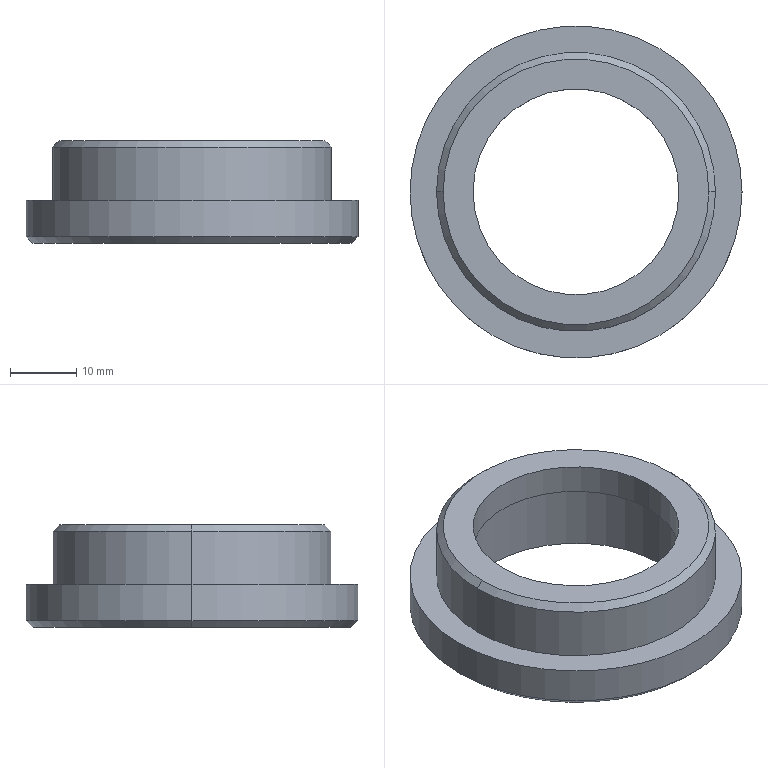Part | SolidWorks | features ICE 4, Chamfer 1, Extrusion 1 | 1 solid | 19 faces | box 50 x 50 x 15.5 mm | volume 11056 mm3 | cylinder 10 | plane 5 | cone 4 | commonest cylinder face diameters 31 x2 33 x2 35 x2 42 x2 50 x2
STEP:
#1=CARTESIAN_POINT('',(-24.,0.,0.));
#2=VERTEX_POINT('',#1);
#3=CARTESIAN_POINT('',(24.,0.,0.));
#4=VERTEX_POINT('',#3);
#5=CARTESIAN_POINT('',(0.,0.,0.));
#6=DIRECTION('',(0.,0.,-1.));
#7=DIRECTION('',(1.,0.,0.));
#8=AXIS2_PLACEMENT_3D('',#5,#6,#7);
#9=CIRCLE('',#8,24.);
#10=EDGE_CURVE('',#2,#4,#9,.T.);
#11=ORIENTED_EDGE('',*,*,#10,.F.);
#12=CARTESIAN_POINT('',(-25.,0.,1.));
#13=VERTEX_POINT('',#12);
#14=CARTESIAN_POINT('',(-25.,0.,1.));
#15=DIRECTION('',(-0.7071,0.,0.7071));
#16=VECTOR('',#15,1000.);
#17=LINE('',#14,#16);
#18=EDGE_CURVE('',#2,#13,#17,.T.);
#19=ORIENTED_EDGE('',*,*,#18,.T.);
#20=CARTESIAN_POINT('',(25.,0.,1.));
#21=VERTEX_POINT('',#20);
#22=CARTESIAN_POINT('',(0.,0.,1.));
#23=DIRECTION('',(0.,0.,1.));
#24=DIRECTION('',(1.,0.,0.));
#25=AXIS2_PLACEMENT_3D('',#22,#23,#24);
#26=CIRCLE('',#25,25.);
#27=EDGE_CURVE('',#21,#13,#26,.T.);
#28=ORIENTED_EDGE('',*,*,#27,.F.);
#29=CARTESIAN_POINT('',(25.,0.,1.));
#30=DIRECTION('',(0.7071,0.,0.7071));
#31=VECTOR('',#30,1000.);
#32=LINE('',#29,#31);
#33=EDGE_CURVE('',#4,#21,#32,.T.);
#34=ORIENTED_EDGE('',*,*,#33,.F.);
#35=EDGE_LOOP('',(#11,#19,#28,#34));
#36=FACE_OUTER_BOUND('',#35,.T.);
#37=CARTESIAN_POINT('',(0.,0.,1.));
#38=DIRECTION('',(0.,0.,1.));
#39=DIRECTION('',(1.,0.,0.));
#40=AXIS2_PLACEMENT_3D('',#37,#38,#39);
#41=CONICAL_SURFACE('',#40,25.,0.7854);
#42=ADVANCED_FACE('',(#36),#41,.T.);
#43=CARTESIAN_POINT('',(20.,0.,15.5));
#44=VERTEX_POINT('',#43);
#45=CARTESIAN_POINT('',(-20.,0.,15.5));
#46=VERTEX_POINT('',#45);
#47=CARTESIAN_POINT('',(0.,0.,15.5));
#48=DIRECTION('',(0.,0.,1.));
#49=DIRECTION('',(1.,0.,0.));
#50=AXIS2_PLACEMENT_3D('',#47,#48,#49);
#51=CIRCLE('',#50,20.);
#52=EDGE_CURVE('',#44,#46,#51,.T.);
#53=ORIENTED_EDGE('',*,*,#52,.F.);
#54=CARTESIAN_POINT('',(21.,0.,14.5));
#55=VERTEX_POINT('',#54);
#56=CARTESIAN_POINT('',(20.,0.,15.5));
#57=DIRECTION('',(0.7071,0.,-0.7071));
#58=VECTOR('',#57,1000.);
#59=LINE('',#56,#58);
#60=EDGE_CURVE('',#44,#55,#59,.T.);
#61=ORIENTED_EDGE('',*,*,#60,.T.);
#62=CARTESIAN_POINT('',(-21.,0.,14.5));
#63=VERTEX_POINT('',#62);
#64=CARTESIAN_POINT('',(0.,0.,14.5));
#65=DIRECTION('',(0.,0.,-1.));
#66=DIRECTION('',(1.,0.,0.));
#67=AXIS2_PLACEMENT_3D('',#64,#65,#66);
#68=CIRCLE('',#67,21.);
#69=EDGE_CURVE('',#63,#55,#68,.T.);
#70=ORIENTED_EDGE('',*,*,#69,.F.);
#71=CARTESIAN_POINT('',(-20.,0.,15.5));
#72=DIRECTION('',(-0.7071,0.,-0.7071));
#73=VECTOR('',#72,1000.);
#74=LINE('',#71,#73);
#75=EDGE_CURVE('',#46,#63,#74,.T.);
#76=ORIENTED_EDGE('',*,*,#75,.F.);
#77=EDGE_LOOP('',(#53,#61,#70,#76));
#78=FACE_OUTER_BOUND('',#77,.T.);
#79=CARTESIAN_POINT('',(0.,0.,15.5));
#80=DIRECTION('',(0.,0.,-1.));
#81=DIRECTION('',(-1.,0.,0.));
#82=AXIS2_PLACEMENT_3D('',#79,#80,#81);
#83=CONICAL_SURFACE('',#82,20.,0.7854);
#84=ADVANCED_FACE('',(#78),#83,.T.);
#85=CARTESIAN_POINT('',(-16.5,0.,11.5));
#86=VERTEX_POINT('',#85);
#87=CARTESIAN_POINT('',(16.5,0.,11.5));
#88=VERTEX_POINT('',#87);
#89=CARTESIAN_POINT('',(0.,0.,11.5));
#90=DIRECTION('',(0.,0.,-1.));
#91=DIRECTION('',(-1.,0.,0.));
#92=AXIS2_PLACEMENT_3D('',#89,#90,#91);
#93=CIRCLE('',#92,16.5);
#94=EDGE_CURVE('',#86,#88,#93,.T.);
#95=ORIENTED_EDGE('',*,*,#94,.T.);
#96=CARTESIAN_POINT('',(16.5,0.,11.));
#97=VERTEX_POINT('',#96);
#98=CARTESIAN_POINT('',(16.5,0.,11.5));
#99=DIRECTION('',(0.,0.,-1.));
#100=VECTOR('',#99,1000.);
#101=LINE('',#98,#100);
#102=EDGE_CURVE('',#88,#97,#101,.T.);
#103=ORIENTED_EDGE('',*,*,#102,.T.);
#104=CARTESIAN_POINT('',(-16.5,0.,11.));
#105=VERTEX_POINT('',#104);
#106=CARTESIAN_POINT('',(0.,0.,11.));
#107=DIRECTION('',(0.,0.,-1.));
#108=DIRECTION('',(-1.,0.,0.));
#109=AXIS2_PLACEMENT_3D('',#106,#107,#108);
#110=CIRCLE('',#109,16.5);
#111=EDGE_CURVE('',#105,#97,#110,.T.);
#112=ORIENTED_EDGE('',*,*,#111,.F.);
#113=CARTESIAN_POINT('',(-16.5,0.,11.5));
#114=DIRECTION('',(0.,0.,-1.));
#115=VECTOR('',#114,1000.);
#116=LINE('',#113,#115);
#117=EDGE_CURVE('',#86,#105,#116,.T.);
#118=ORIENTED_EDGE('',*,*,#117,.F.);
#119=EDGE_LOOP('',(#95,#103,#112,#118));
#120=FACE_OUTER_BOUND('',#119,.T.);
#121=CARTESIAN_POINT('',(0.,0.,11.5));
#122=DIRECTION('',(0.,0.,-1.));
#123=DIRECTION('',(-1.,0.,0.));
#124=AXIS2_PLACEMENT_3D('',#121,#122,#123);
#125=CYLINDRICAL_SURFACE('',#124,16.5);
#126=ADVANCED_FACE('',(#120),#125,.T.);
#127=CARTESIAN_POINT('',(17.5,0.,11.5));
#128=VERTEX_POINT('',#127);
#129=CARTESIAN_POINT('',(-17.5,0.,11.5));
#130=VERTEX_POINT('',#129);
#131=CARTESIAN_POINT('',(0.,0.,11.5));
#132=DIRECTION('',(0.,0.,-1.));
#133=DIRECTION('',(-1.,0.,0.));
#134=AXIS2_PLACEMENT_3D('',#131,#132,#133);
#135=CIRCLE('',#134,17.5);
#136=EDGE_CURVE('',#128,#130,#135,.T.);
#137=ORIENTED_EDGE('',*,*,#136,.F.);
#138=CARTESIAN_POINT('',(17.5,0.,0.));
#139=VERTEX_POINT('',#138);
#140=CARTESIAN_POINT('',(17.5,0.,11.));
#141=DIRECTION('',(0.,0.,-1.));
#142=VECTOR('',#141,1000.);
#143=LINE('',#140,#142);
#144=EDGE_CURVE('',#128,#139,#143,.T.);
#145=ORIENTED_EDGE('',*,*,#144,.T.);
#146=CARTESIAN_POINT('',(-17.5,0.,0.));
#147=VERTEX_POINT('',#146);
#148=CARTESIAN_POINT('',(0.,0.,0.));
#149=DIRECTION('',(0.,0.,-1.));
#150=DIRECTION('',(-1.,0.,0.));
#151=AXIS2_PLACEMENT_3D('',#148,#149,#150);
#152=CIRCLE('',#151,17.5);
#153=EDGE_CURVE('',#139,#147,#152,.T.);
#154=ORIENTED_EDGE('',*,*,#153,.T.);
#155=CARTESIAN_POINT('',(-17.5,0.,11.));
#156=DIRECTION('',(0.,0.,-1.));
#157=VECTOR('',#156,1000.);
#158=LINE('',#155,#157);
#159=EDGE_CURVE('',#130,#147,#158,.T.);
#160=ORIENTED_EDGE('',*,*,#159,.F.);
#161=EDGE_LOOP('',(#137,#145,#154,#160));
#162=FACE_OUTER_BOUND('',#161,.T.);
#163=CARTESIAN_POINT('',(0.,0.,11.));
#164=DIRECTION('',(0.,0.,-1.));
#165=DIRECTION('',(-1.,0.,0.));
#166=AXIS2_PLACEMENT_3D('',#163,#164,#165);
#167=CYLINDRICAL_SURFACE('',#166,17.5);
#168=ADVANCED_FACE('',(#162),#167,.F.);
#169=ORIENTED_EDGE('',*,*,#69,.T.);
#170=CARTESIAN_POINT('',(21.,0.,6.5));
#171=VERTEX_POINT('',#170);
#172=CARTESIAN_POINT('',(21.,0.,15.5));
#173=DIRECTION('',(0.,0.,-1.));
#174=VECTOR('',#173,1000.);
#175=LINE('',#172,#174);
#176=EDGE_CURVE('',#55,#171,#175,.T.);
#177=ORIENTED_EDGE('',*,*,#176,.T.);
#178=CARTESIAN_POINT('',(-21.,0.,6.5));
#179=VERTEX_POINT('',#178);
#180=CARTESIAN_POINT('',(0.,0.,6.5));
#181=DIRECTION('',(0.,0.,1.));
#182=DIRECTION('',(1.,0.,0.));
#183=AXIS2_PLACEMENT_3D('',#180,#181,#182);
#184=CIRCLE('',#183,21.);
#185=EDGE_CURVE('',#171,#179,#184,.T.);
#186=ORIENTED_EDGE('',*,*,#185,.T.);
#187=CARTESIAN_POINT('',(-21.,0.,15.5));
#188=DIRECTION('',(0.,0.,-1.));
#189=VECTOR('',#188,1000.);
#190=LINE('',#187,#189);
#191=EDGE_CURVE('',#63,#179,#190,.T.);
#192=ORIENTED_EDGE('',*,*,#191,.F.);
#193=EDGE_LOOP('',(#169,#177,#186,#192));
#194=FACE_OUTER_BOUND('',#193,.T.);
#195=CARTESIAN_POINT('',(0.,0.,15.5));
#196=DIRECTION('',(0.,0.,-1.));
#197=DIRECTION('',(-1.,0.,0.));
#198=AXIS2_PLACEMENT_3D('',#195,#196,#197);
#199=CYLINDRICAL_SURFACE('',#198,21.);
#200=ADVANCED_FACE('',(#194),#199,.T.);
#201=CARTESIAN_POINT('',(25.,0.,6.5));
#202=VERTEX_POINT('',#201);
#203=CARTESIAN_POINT('',(-25.,0.,6.5));
#204=VERTEX_POINT('',#203);
#205=CARTESIAN_POINT('',(0.,0.,6.5));
#206=DIRECTION('',(0.,0.,1.));
#207=DIRECTION('',(1.,0.,0.));
#208=AXIS2_PLACEMENT_3D('',#205,#206,#207);
#209=CIRCLE('',#208,25.);
#210=EDGE_CURVE('',#202,#204,#209,.T.);
#211=ORIENTED_EDGE('',*,*,#210,.F.);
#212=CARTESIAN_POINT('',(25.,0.,6.5));
#213=DIRECTION('',(0.,0.,-1.));
#214=VECTOR('',#213,1000.);
#215=LINE('',#212,#214);
#216=EDGE_CURVE('',#202,#21,#215,.T.);
#217=ORIENTED_EDGE('',*,*,#216,.T.);
#218=ORIENTED_EDGE('',*,*,#27,.T.);
#219=CARTESIAN_POINT('',(-25.,0.,6.5));
#220=DIRECTION('',(0.,0.,-1.));
#221=VECTOR('',#220,1000.);
#222=LINE('',#219,#221);
#223=EDGE_CURVE('',#204,#13,#222,.T.);
#224=ORIENTED_EDGE('',*,*,#223,.F.);
#225=EDGE_LOOP('',(#211,#217,#218,#224));
#226=FACE_OUTER_BOUND('',#225,.T.);
#227=CARTESIAN_POINT('',(0.,0.,6.5));
#228=DIRECTION('',(0.,0.,-1.));
#229=DIRECTION('',(-1.,0.,0.));
#230=AXIS2_PLACEMENT_3D('',#227,#228,#229);
#231=CYLINDRICAL_SURFACE('',#230,25.);
#232=ADVANCED_FACE('',(#226),#231,.T.);
#233=CARTESIAN_POINT('',(-15.5,0.,11.));
#234=VERTEX_POINT('',#233);
#235=CARTESIAN_POINT('',(15.5,0.,11.));
#236=VERTEX_POINT('',#235);
#237=CARTESIAN_POINT('',(0.,0.,11.));
#238=DIRECTION('',(0.,0.,1.));
#239=DIRECTION('',(-1.,0.,0.));
#240=AXIS2_PLACEMENT_3D('',#237,#238,#239);
#241=CIRCLE('',#240,15.5);
#242=EDGE_CURVE('',#234,#236,#241,.T.);
#243=ORIENTED_EDGE('',*,*,#242,.F.);
#244=CARTESIAN_POINT('',(-15.5,0.,15.5));
#245=VERTEX_POINT('',#244);
#246=CARTESIAN_POINT('',(-15.5,0.,-27.5));
#247=DIRECTION('',(0.,0.,1.));
#248=VECTOR('',#247,1000.);
#249=LINE('',#246,#248);
#250=EDGE_CURVE('',#234,#245,#249,.T.);
#251=ORIENTED_EDGE('',*,*,#250,.T.);
#252=CARTESIAN_POINT('',(15.5,0.,15.5));
#253=VERTEX_POINT('',#252);
#254=CARTESIAN_POINT('',(0.,0.,15.5));
#255=DIRECTION('',(0.,0.,1.));
#256=DIRECTION('',(1.,0.,0.));
#257=AXIS2_PLACEMENT_3D('',#254,#255,#256);
#258=CIRCLE('',#257,15.5);
#259=EDGE_CURVE('',#245,#253,#258,.T.);
#260=ORIENTED_EDGE('',*,*,#259,.T.);
#261=CARTESIAN_POINT('',(15.5,0.,-27.5));
#262=DIRECTION('',(0.,0.,1.));
#263=VECTOR('',#262,1000.);
#264=LINE('',#261,#263);
#265=EDGE_CURVE('',#236,#253,#264,.T.);
#266=ORIENTED_EDGE('',*,*,#265,.F.);
#267=EDGE_LOOP('',(#243,#251,#260,#266));
#268=FACE_OUTER_BOUND('',#267,.T.);
#269=CARTESIAN_POINT('',(0.,0.,-27.5));
#270=DIRECTION('',(0.,0.,1.));
#271=DIRECTION('',(1.,0.,0.));
#272=AXIS2_PLACEMENT_3D('',#269,#270,#271);
#273=CYLINDRICAL_SURFACE('',#272,15.5);
#274=ADVANCED_FACE('',(#268),#273,.F.);
#275=CARTESIAN_POINT('',(0.,0.,11.));
#276=DIRECTION('',(0.,0.,1.));
#277=DIRECTION('',(-1.,0.,0.));
#278=AXIS2_PLACEMENT_3D('',#275,#276,#277);
#279=CIRCLE('',#278,15.5);
#280=EDGE_CURVE('',#236,#234,#279,.T.);
#281=ORIENTED_EDGE('',*,*,#280,.T.);
#282=ORIENTED_EDGE('',*,*,#242,.T.);
#283=EDGE_LOOP('',(#281,#282));
#284=FACE_BOUND('',#283,.T.);
#285=ORIENTED_EDGE('',*,*,#111,.T.);
#286=CARTESIAN_POINT('',(0.,0.,11.));
#287=DIRECTION('',(0.,0.,-1.));
#288=DIRECTION('',(-1.,0.,0.));
#289=AXIS2_PLACEMENT_3D('',#286,#287,#288);
#290=CIRCLE('',#289,16.5);
#291=EDGE_CURVE('',#97,#105,#290,.T.);
#292=ORIENTED_EDGE('',*,*,#291,.T.);
#293=EDGE_LOOP('',(#285,#292));
#294=FACE_OUTER_BOUND('',#293,.T.);
#295=CARTESIAN_POINT('',(0.,0.,11.));
#296=DIRECTION('',(0.,0.,-1.));
#297=DIRECTION('',(-1.,0.,0.));
#298=AXIS2_PLACEMENT_3D('',#295,#296,#297);
#299=PLANE('',#298);
#300=ADVANCED_FACE('',(#284,#294),#299,.T.);
#301=ORIENTED_EDGE('',*,*,#250,.F.);
#302=ORIENTED_EDGE('',*,*,#280,.F.);
#303=ORIENTED_EDGE('',*,*,#265,.T.);
#304=CARTESIAN_POINT('',(0.,0.,15.5));
#305=DIRECTION('',(0.,0.,1.));
#306=DIRECTION('',(1.,0.,0.));
#307=AXIS2_PLACEMENT_3D('',#304,#305,#306);
#308=CIRCLE('',#307,15.5);
#309=EDGE_CURVE('',#253,#245,#308,.T.);
#310=ORIENTED_EDGE('',*,*,#309,.T.);
#311=EDGE_LOOP('',(#301,#302,#303,#310));
#312=FACE_OUTER_BOUND('',#311,.T.);
#313=CARTESIAN_POINT('',(0.,0.,-27.5));
#314=DIRECTION('',(0.,0.,1.));
#315=DIRECTION('',(1.,0.,0.));
#316=AXIS2_PLACEMENT_3D('',#313,#314,#315);
#317=CYLINDRICAL_SURFACE('',#316,15.5);
#318=ADVANCED_FACE('',(#312),#317,.F.);
#319=ORIENTED_EDGE('',*,*,#216,.F.);
#320=CARTESIAN_POINT('',(0.,0.,6.5));
#321=DIRECTION('',(0.,0.,1.));
#322=DIRECTION('',(1.,0.,0.));
#323=AXIS2_PLACEMENT_3D('',#320,#321,#322);
#324=CIRCLE('',#323,25.);
#325=EDGE_CURVE('',#204,#202,#324,.T.);
#326=ORIENTED_EDGE('',*,*,#325,.F.);
#327=ORIENTED_EDGE('',*,*,#223,.T.);
#328=CARTESIAN_POINT('',(0.,0.,1.));
#329=DIRECTION('',(0.,0.,1.));
#330=DIRECTION('',(1.,0.,0.));
#331=AXIS2_PLACEMENT_3D('',#328,#329,#330);
#332=CIRCLE('',#331,25.);
#333=EDGE_CURVE('',#13,#21,#332,.T.);
#334=ORIENTED_EDGE('',*,*,#333,.T.);
#335=EDGE_LOOP('',(#319,#326,#327,#334));
#336=FACE_OUTER_BOUND('',#335,.T.);
#337=CARTESIAN_POINT('',(0.,0.,6.5));
#338=DIRECTION('',(0.,0.,-1.));
#339=DIRECTION('',(-1.,0.,0.));
#340=AXIS2_PLACEMENT_3D('',#337,#338,#339);
#341=CYLINDRICAL_SURFACE('',#340,25.);
#342=ADVANCED_FACE('',(#336),#341,.T.);
#343=CARTESIAN_POINT('',(0.,0.,6.5));
#344=DIRECTION('',(0.,0.,1.));
#345=DIRECTION('',(1.,0.,0.));
#346=AXIS2_PLACEMENT_3D('',#343,#344,#345);
#347=CIRCLE('',#346,21.);
#348=EDGE_CURVE('',#179,#171,#347,.T.);
#349=ORIENTED_EDGE('',*,*,#348,.F.);
#350=ORIENTED_EDGE('',*,*,#185,.F.);
#351=EDGE_LOOP('',(#349,#350));
#352=FACE_BOUND('',#351,.T.);
#353=ORIENTED_EDGE('',*,*,#325,.T.);
#354=ORIENTED_EDGE('',*,*,#210,.T.);
#355=EDGE_LOOP('',(#353,#354));
#356=FACE_OUTER_BOUND('',#355,.T.);
#357=CARTESIAN_POINT('',(0.,0.,6.5));
#358=DIRECTION('',(0.,0.,1.));
#359=DIRECTION('',(1.,0.,0.));
#360=AXIS2_PLACEMENT_3D('',#357,#358,#359);
#361=PLANE('',#360);
#362=ADVANCED_FACE('',(#352,#356),#361,.T.);
#363=CARTESIAN_POINT('',(0.,0.,0.));
#364=DIRECTION('',(0.,0.,-1.));
#365=DIRECTION('',(1.,0.,0.));
#366=AXIS2_PLACEMENT_3D('',#363,#364,#365);
#367=CIRCLE('',#366,24.);
#368=EDGE_CURVE('',#4,#2,#367,.T.);
#369=ORIENTED_EDGE('',*,*,#368,.T.);
#370=ORIENTED_EDGE('',*,*,#10,.T.);
#371=EDGE_LOOP('',(#369,#370));
#372=FACE_OUTER_BOUND('',#371,.T.);
#373=CARTESIAN_POINT('',(0.,0.,0.));
#374=DIRECTION('',(0.,0.,-1.));
#375=DIRECTION('',(-1.,0.,0.));
#376=AXIS2_PLACEMENT_3D('',#373,#374,#375);
#377=CIRCLE('',#376,17.5);
#378=EDGE_CURVE('',#147,#139,#377,.T.);
#379=ORIENTED_EDGE('',*,*,#378,.F.);
#380=ORIENTED_EDGE('',*,*,#153,.F.);
#381=EDGE_LOOP('',(#379,#380));
#382=FACE_BOUND('',#381,.T.);
#383=CARTESIAN_POINT('',(0.,0.,0.));
#384=DIRECTION('',(0.,0.,1.));
#385=DIRECTION('',(1.,0.,0.));
#386=AXIS2_PLACEMENT_3D('',#383,#384,#385);
#387=PLANE('',#386);
#388=ADVANCED_FACE('',(#372,#382),#387,.F.);
#389=ORIENTED_EDGE('',*,*,#176,.F.);
#390=CARTESIAN_POINT('',(0.,0.,14.5));
#391=DIRECTION('',(0.,0.,-1.));
#392=DIRECTION('',(1.,0.,0.));
#393=AXIS2_PLACEMENT_3D('',#390,#391,#392);
#394=CIRCLE('',#393,21.);
#395=EDGE_CURVE('',#55,#63,#394,.T.);
#396=ORIENTED_EDGE('',*,*,#395,.T.);
#397=ORIENTED_EDGE('',*,*,#191,.T.);
#398=ORIENTED_EDGE('',*,*,#348,.T.);
#399=EDGE_LOOP('',(#389,#396,#397,#398));
#400=FACE_OUTER_BOUND('',#399,.T.);
#401=CARTESIAN_POINT('',(0.,0.,15.5));
#402=DIRECTION('',(0.,0.,-1.));
#403=DIRECTION('',(-1.,0.,0.));
#404=AXIS2_PLACEMENT_3D('',#401,#402,#403);
#405=CYLINDRICAL_SURFACE('',#404,21.);
#406=ADVANCED_FACE('',(#400),#405,.T.);
#407=CARTESIAN_POINT('',(0.,0.,15.5));
#408=DIRECTION('',(0.,0.,1.));
#409=DIRECTION('',(1.,0.,0.));
#410=AXIS2_PLACEMENT_3D('',#407,#408,#409);
#411=CIRCLE('',#410,20.);
#412=EDGE_CURVE('',#46,#44,#411,.T.);
#413=ORIENTED_EDGE('',*,*,#412,.T.);
#414=ORIENTED_EDGE('',*,*,#52,.T.);
#415=EDGE_LOOP('',(#413,#414));
#416=FACE_OUTER_BOUND('',#415,.T.);
#417=ORIENTED_EDGE('',*,*,#309,.F.);
#418=ORIENTED_EDGE('',*,*,#259,.F.);
#419=EDGE_LOOP('',(#417,#418));
#420=FACE_BOUND('',#419,.T.);
#421=CARTESIAN_POINT('',(0.,0.,15.5));
#422=DIRECTION('',(0.,0.,1.));
#423=DIRECTION('',(1.,0.,0.));
#424=AXIS2_PLACEMENT_3D('',#421,#422,#423);
#425=PLANE('',#424);
#426=ADVANCED_FACE('',(#416,#420),#425,.T.);
#427=ORIENTED_EDGE('',*,*,#144,.F.);
#428=CARTESIAN_POINT('',(0.,0.,11.5));
#429=DIRECTION('',(0.,0.,-1.));
#430=DIRECTION('',(-1.,0.,0.));
#431=AXIS2_PLACEMENT_3D('',#428,#429,#430);
#432=CIRCLE('',#431,17.5);
#433=EDGE_CURVE('',#130,#128,#432,.T.);
#434=ORIENTED_EDGE('',*,*,#433,.F.);
#435=ORIENTED_EDGE('',*,*,#159,.T.);
#436=ORIENTED_EDGE('',*,*,#378,.T.);
#437=EDGE_LOOP('',(#427,#434,#435,#436));
#438=FACE_OUTER_BOUND('',#437,.T.);
#439=CARTESIAN_POINT('',(0.,0.,11.));
#440=DIRECTION('',(0.,0.,-1.));
#441=DIRECTION('',(-1.,0.,0.));
#442=AXIS2_PLACEMENT_3D('',#439,#440,#441);
#443=CYLINDRICAL_SURFACE('',#442,17.5);
#444=ADVANCED_FACE('',(#438),#443,.F.);
#445=ORIENTED_EDGE('',*,*,#94,.F.);
#446=CARTESIAN_POINT('',(0.,0.,11.5));
#447=DIRECTION('',(0.,0.,-1.));
#448=DIRECTION('',(-1.,0.,0.));
#449=AXIS2_PLACEMENT_3D('',#446,#447,#448);
#450=CIRCLE('',#449,16.5);
#451=EDGE_CURVE('',#88,#86,#450,.T.);
#452=ORIENTED_EDGE('',*,*,#451,.F.);
#453=EDGE_LOOP('',(#445,#452));
#454=FACE_BOUND('',#453,.T.);
#455=ORIENTED_EDGE('',*,*,#433,.T.);
#456=ORIENTED_EDGE('',*,*,#136,.T.);
#457=EDGE_LOOP('',(#455,#456));
#458=FACE_OUTER_BOUND('',#457,.T.);
#459=CARTESIAN_POINT('',(0.,0.,11.5));
#460=DIRECTION('',(0.,0.,-1.));
#461=DIRECTION('',(-1.,0.,0.));
#462=AXIS2_PLACEMENT_3D('',#459,#460,#461);
#463=PLANE('',#462);
#464=ADVANCED_FACE('',(#454,#458),#463,.T.);
#465=ORIENTED_EDGE('',*,*,#102,.F.);
#466=ORIENTED_EDGE('',*,*,#451,.T.);
#467=ORIENTED_EDGE('',*,*,#117,.T.);
#468=ORIENTED_EDGE('',*,*,#291,.F.);
#469=EDGE_LOOP('',(#465,#466,#467,#468));
#470=FACE_OUTER_BOUND('',#469,.T.);
#471=CARTESIAN_POINT('',(0.,0.,11.5));
#472=DIRECTION('',(0.,0.,-1.));
#473=DIRECTION('',(-1.,0.,0.));
#474=AXIS2_PLACEMENT_3D('',#471,#472,#473);
#475=CYLINDRICAL_SURFACE('',#474,16.5);
#476=ADVANCED_FACE('',(#470),#475,.T.);
#477=ORIENTED_EDGE('',*,*,#60,.F.);
#478=ORIENTED_EDGE('',*,*,#412,.F.);
#479=ORIENTED_EDGE('',*,*,#75,.T.);
#480=ORIENTED_EDGE('',*,*,#395,.F.);
#481=EDGE_LOOP('',(#477,#478,#479,#480));
#482=FACE_OUTER_BOUND('',#481,.T.);
#483=CARTESIAN_POINT('',(0.,0.,15.5));
#484=DIRECTION('',(0.,0.,-1.));
#485=DIRECTION('',(-1.,0.,0.));
#486=AXIS2_PLACEMENT_3D('',#483,#484,#485);
#487=CONICAL_SURFACE('',#486,20.,0.7854);
#488=ADVANCED_FACE('',(#482),#487,.T.);
#489=ORIENTED_EDGE('',*,*,#18,.F.);
#490=ORIENTED_EDGE('',*,*,#368,.F.);
#491=ORIENTED_EDGE('',*,*,#33,.T.);
#492=ORIENTED_EDGE('',*,*,#333,.F.);
#493=EDGE_LOOP('',(#489,#490,#491,#492));
#494=FACE_OUTER_BOUND('',#493,.T.);
#495=CARTESIAN_POINT('',(0.,0.,1.));
#496=DIRECTION('',(0.,0.,1.));
#497=DIRECTION('',(1.,0.,0.));
#498=AXIS2_PLACEMENT_3D('',#495,#496,#497);
#499=CONICAL_SURFACE('',#498,25.,0.7854);
#500=ADVANCED_FACE('',(#494),#499,.T.);
#501=CLOSED_SHELL('',(#42,#84,#126,#168,#200,#232,#274,#300,#318,#342,#362,#388,#406,#426,#444,#464,#476,#488,#500));
#502=MANIFOLD_SOLID_BREP('',#501);
#503=CARTESIAN_POINT('',(0.,0.,0.));
#504=DIRECTION('',(0.,0.,1.));
#505=DIRECTION('',(1.,0.,0.));
#506=AXIS2_PLACEMENT_3D('',#503,#504,#505);
#507=(LENGTH_UNIT()NAMED_UNIT(*)SI_UNIT(.MILLI.,.METRE.));
#508=UNCERTAINTY_MEASURE_WITH_UNIT(LENGTH_MEASURE(0.00001),#507,'','');
#509=(NAMED_UNIT(*)PLANE_ANGLE_UNIT()SI_UNIT($,.RADIAN.));
#510=(NAMED_UNIT(*)SI_UNIT($,.STERADIAN.)SOLID_ANGLE_UNIT());
#511=(GEOMETRIC_REPRESENTATION_CONTEXT(3)GLOBAL_UNCERTAINTY_ASSIGNED_CONTEXT((#508))GLOBAL_UNIT_ASSIGNED_CONTEXT((#507,#509,#510))REPRESENTATION_CONTEXT('',''));
#512=ADVANCED_BREP_SHAPE_REPRESENTATION('',(#502,#506),#511);